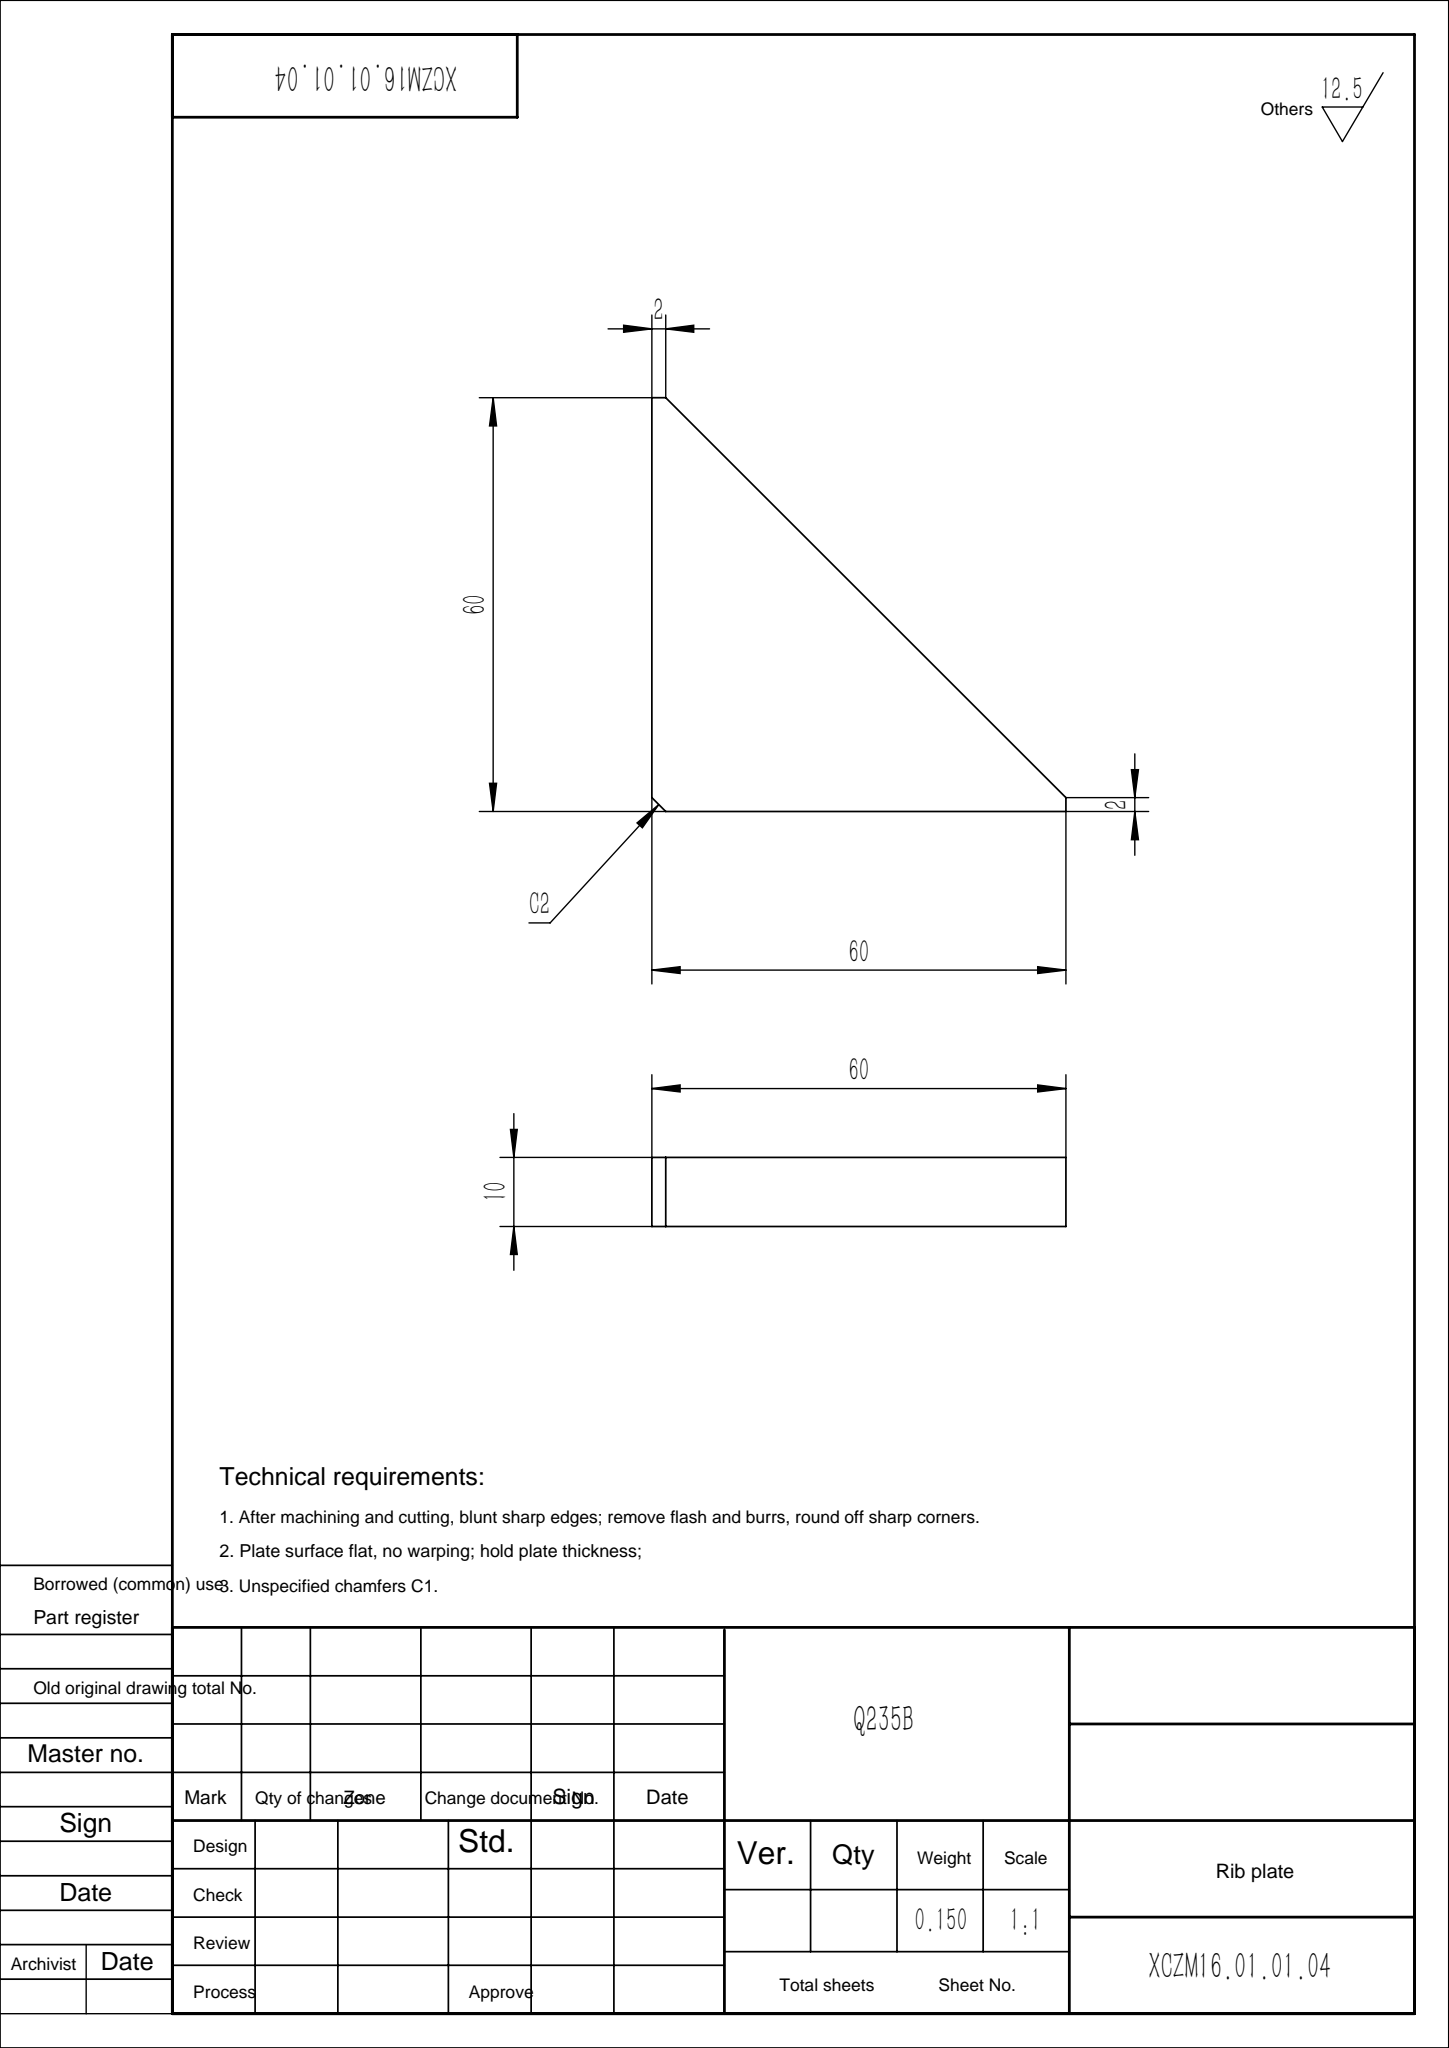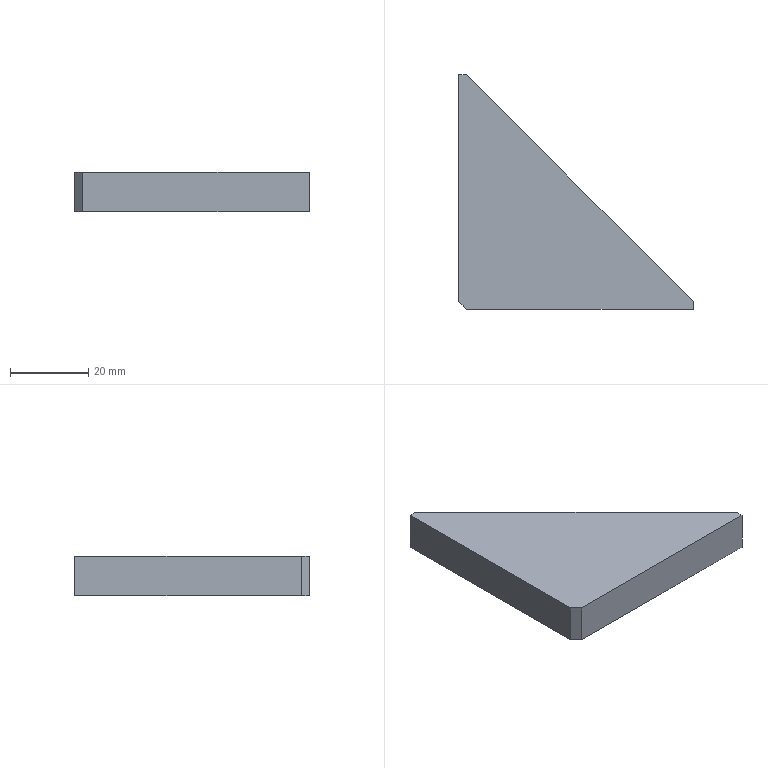Part | SolidWorks | features Chamfer 1, Extrusion 1 | 1 solid | 8 faces | box 60 x 60 x 10 mm | volume 19160 mm3 | plane 8
STEP:
#1=CARTESIAN_POINT('',(2.,60.,0.));
#2=VERTEX_POINT('',#1);
#3=CARTESIAN_POINT('',(0.,60.,0.));
#4=VERTEX_POINT('',#3);
#5=CARTESIAN_POINT('',(2.,60.,0.));
#6=DIRECTION('',(-1.,0.,0.));
#7=VECTOR('',#6,1000.);
#8=LINE('',#5,#7);
#9=EDGE_CURVE('',#2,#4,#8,.T.);
#10=ORIENTED_EDGE('',*,*,#9,.T.);
#11=CARTESIAN_POINT('',(0.,60.,10.));
#12=VERTEX_POINT('',#11);
#13=CARTESIAN_POINT('',(0.,60.,10.));
#14=DIRECTION('',(0.,0.,-1.));
#15=VECTOR('',#14,1000.);
#16=LINE('',#13,#15);
#17=EDGE_CURVE('',#12,#4,#16,.T.);
#18=ORIENTED_EDGE('',*,*,#17,.F.);
#19=CARTESIAN_POINT('',(2.,60.,10.));
#20=VERTEX_POINT('',#19);
#21=CARTESIAN_POINT('',(2.,60.,10.));
#22=DIRECTION('',(-1.,0.,0.));
#23=VECTOR('',#22,1000.);
#24=LINE('',#21,#23);
#25=EDGE_CURVE('',#20,#12,#24,.T.);
#26=ORIENTED_EDGE('',*,*,#25,.F.);
#27=CARTESIAN_POINT('',(2.,60.,10.));
#28=DIRECTION('',(0.,0.,-1.));
#29=VECTOR('',#28,1000.);
#30=LINE('',#27,#29);
#31=EDGE_CURVE('',#20,#2,#30,.T.);
#32=ORIENTED_EDGE('',*,*,#31,.T.);
#33=EDGE_LOOP('',(#10,#18,#26,#32));
#34=FACE_OUTER_BOUND('',#33,.T.);
#35=CARTESIAN_POINT('',(2.,60.,10.));
#36=DIRECTION('',(0.,-1.,0.));
#37=DIRECTION('',(0.,0.,-1.));
#38=AXIS2_PLACEMENT_3D('',#35,#36,#37);
#39=PLANE('',#38);
#40=ADVANCED_FACE('',(#34),#39,.F.);
#41=CARTESIAN_POINT('',(0.,2.,0.));
#42=VERTEX_POINT('',#41);
#43=CARTESIAN_POINT('',(0.,60.,0.));
#44=DIRECTION('',(0.,-1.,0.));
#45=VECTOR('',#44,1000.);
#46=LINE('',#43,#45);
#47=EDGE_CURVE('',#4,#42,#46,.T.);
#48=ORIENTED_EDGE('',*,*,#47,.T.);
#49=CARTESIAN_POINT('',(0.,2.,10.));
#50=VERTEX_POINT('',#49);
#51=CARTESIAN_POINT('',(0.,2.,10.));
#52=DIRECTION('',(0.,0.,1.));
#53=VECTOR('',#52,1000.);
#54=LINE('',#51,#53);
#55=EDGE_CURVE('',#42,#50,#54,.T.);
#56=ORIENTED_EDGE('',*,*,#55,.T.);
#57=CARTESIAN_POINT('',(0.,60.,10.));
#58=DIRECTION('',(0.,-1.,0.));
#59=VECTOR('',#58,1000.);
#60=LINE('',#57,#59);
#61=EDGE_CURVE('',#12,#50,#60,.T.);
#62=ORIENTED_EDGE('',*,*,#61,.F.);
#63=ORIENTED_EDGE('',*,*,#17,.T.);
#64=EDGE_LOOP('',(#48,#56,#62,#63));
#65=FACE_OUTER_BOUND('',#64,.T.);
#66=CARTESIAN_POINT('',(0.,60.,10.));
#67=DIRECTION('',(1.,0.,0.));
#68=DIRECTION('',(0.,1.,0.));
#69=AXIS2_PLACEMENT_3D('',#66,#67,#68);
#70=PLANE('',#69);
#71=ADVANCED_FACE('',(#65),#70,.F.);
#72=CARTESIAN_POINT('',(2.,0.,10.));
#73=VERTEX_POINT('',#72);
#74=CARTESIAN_POINT('',(60.,0.,10.));
#75=VERTEX_POINT('',#74);
#76=CARTESIAN_POINT('',(0.,0.,10.));
#77=DIRECTION('',(1.,0.,0.));
#78=VECTOR('',#77,1000.);
#79=LINE('',#76,#78);
#80=EDGE_CURVE('',#73,#75,#79,.T.);
#81=ORIENTED_EDGE('',*,*,#80,.F.);
#82=CARTESIAN_POINT('',(2.,0.,0.));
#83=VERTEX_POINT('',#82);
#84=CARTESIAN_POINT('',(2.,0.,10.));
#85=DIRECTION('',(0.,0.,-1.));
#86=VECTOR('',#85,1000.);
#87=LINE('',#84,#86);
#88=EDGE_CURVE('',#73,#83,#87,.T.);
#89=ORIENTED_EDGE('',*,*,#88,.T.);
#90=CARTESIAN_POINT('',(60.,0.,0.));
#91=VERTEX_POINT('',#90);
#92=CARTESIAN_POINT('',(0.,0.,0.));
#93=DIRECTION('',(1.,0.,0.));
#94=VECTOR('',#93,1000.);
#95=LINE('',#92,#94);
#96=EDGE_CURVE('',#83,#91,#95,.T.);
#97=ORIENTED_EDGE('',*,*,#96,.T.);
#98=CARTESIAN_POINT('',(60.,0.,10.));
#99=DIRECTION('',(0.,0.,-1.));
#100=VECTOR('',#99,1000.);
#101=LINE('',#98,#100);
#102=EDGE_CURVE('',#75,#91,#101,.T.);
#103=ORIENTED_EDGE('',*,*,#102,.F.);
#104=EDGE_LOOP('',(#81,#89,#97,#103));
#105=FACE_OUTER_BOUND('',#104,.T.);
#106=CARTESIAN_POINT('',(0.,0.,10.));
#107=DIRECTION('',(0.,1.,0.));
#108=DIRECTION('',(0.,0.,1.));
#109=AXIS2_PLACEMENT_3D('',#106,#107,#108);
#110=PLANE('',#109);
#111=ADVANCED_FACE('',(#105),#110,.F.);
#112=CARTESIAN_POINT('',(60.,2.,0.));
#113=VERTEX_POINT('',#112);
#114=CARTESIAN_POINT('',(60.,0.,0.));
#115=DIRECTION('',(0.,1.,0.));
#116=VECTOR('',#115,1000.);
#117=LINE('',#114,#116);
#118=EDGE_CURVE('',#91,#113,#117,.T.);
#119=ORIENTED_EDGE('',*,*,#118,.T.);
#120=CARTESIAN_POINT('',(60.,2.,10.));
#121=VERTEX_POINT('',#120);
#122=CARTESIAN_POINT('',(60.,2.,10.));
#123=DIRECTION('',(0.,0.,-1.));
#124=VECTOR('',#123,1000.);
#125=LINE('',#122,#124);
#126=EDGE_CURVE('',#121,#113,#125,.T.);
#127=ORIENTED_EDGE('',*,*,#126,.F.);
#128=CARTESIAN_POINT('',(60.,0.,10.));
#129=DIRECTION('',(0.,1.,0.));
#130=VECTOR('',#129,1000.);
#131=LINE('',#128,#130);
#132=EDGE_CURVE('',#75,#121,#131,.T.);
#133=ORIENTED_EDGE('',*,*,#132,.F.);
#134=ORIENTED_EDGE('',*,*,#102,.T.);
#135=EDGE_LOOP('',(#119,#127,#133,#134));
#136=FACE_OUTER_BOUND('',#135,.T.);
#137=CARTESIAN_POINT('',(60.,0.,10.));
#138=DIRECTION('',(-1.,0.,0.));
#139=DIRECTION('',(0.,0.,1.));
#140=AXIS2_PLACEMENT_3D('',#137,#138,#139);
#141=PLANE('',#140);
#142=ADVANCED_FACE('',(#136),#141,.F.);
#143=CARTESIAN_POINT('',(60.,2.,0.));
#144=DIRECTION('',(-0.7071,0.7071,0.));
#145=VECTOR('',#144,1000.);
#146=LINE('',#143,#145);
#147=EDGE_CURVE('',#113,#2,#146,.T.);
#148=ORIENTED_EDGE('',*,*,#147,.T.);
#149=ORIENTED_EDGE('',*,*,#31,.F.);
#150=CARTESIAN_POINT('',(60.,2.,10.));
#151=DIRECTION('',(-0.7071,0.7071,0.));
#152=VECTOR('',#151,1000.);
#153=LINE('',#150,#152);
#154=EDGE_CURVE('',#121,#20,#153,.T.);
#155=ORIENTED_EDGE('',*,*,#154,.F.);
#156=ORIENTED_EDGE('',*,*,#126,.T.);
#157=EDGE_LOOP('',(#148,#149,#155,#156));
#158=FACE_OUTER_BOUND('',#157,.T.);
#159=CARTESIAN_POINT('',(60.,2.,10.));
#160=DIRECTION('',(-0.7071,-0.7071,0.));
#161=DIRECTION('',(0.7071,-0.7071,0.));
#162=AXIS2_PLACEMENT_3D('',#159,#160,#161);
#163=PLANE('',#162);
#164=ADVANCED_FACE('',(#158),#163,.F.);
#165=ORIENTED_EDGE('',*,*,#61,.T.);
#166=CARTESIAN_POINT('',(1.,1.,10.));
#167=DIRECTION('',(0.7071,-0.7071,0.));
#168=VECTOR('',#167,1000.);
#169=LINE('',#166,#168);
#170=EDGE_CURVE('',#50,#73,#169,.T.);
#171=ORIENTED_EDGE('',*,*,#170,.T.);
#172=ORIENTED_EDGE('',*,*,#80,.T.);
#173=ORIENTED_EDGE('',*,*,#132,.T.);
#174=ORIENTED_EDGE('',*,*,#154,.T.);
#175=ORIENTED_EDGE('',*,*,#25,.T.);
#176=EDGE_LOOP('',(#165,#171,#172,#173,#174,#175));
#177=FACE_OUTER_BOUND('',#176,.T.);
#178=CARTESIAN_POINT('',(0.,0.,10.));
#179=DIRECTION('',(0.,0.,1.));
#180=DIRECTION('',(1.,0.,0.));
#181=AXIS2_PLACEMENT_3D('',#178,#179,#180);
#182=PLANE('',#181);
#183=ADVANCED_FACE('',(#177),#182,.T.);
#184=ORIENTED_EDGE('',*,*,#96,.F.);
#185=CARTESIAN_POINT('',(2.,0.,0.));
#186=DIRECTION('',(-0.7071,0.7071,0.));
#187=VECTOR('',#186,1000.);
#188=LINE('',#185,#187);
#189=EDGE_CURVE('',#83,#42,#188,.T.);
#190=ORIENTED_EDGE('',*,*,#189,.T.);
#191=ORIENTED_EDGE('',*,*,#47,.F.);
#192=ORIENTED_EDGE('',*,*,#9,.F.);
#193=ORIENTED_EDGE('',*,*,#147,.F.);
#194=ORIENTED_EDGE('',*,*,#118,.F.);
#195=EDGE_LOOP('',(#184,#190,#191,#192,#193,#194));
#196=FACE_OUTER_BOUND('',#195,.T.);
#197=CARTESIAN_POINT('',(0.,0.,0.));
#198=DIRECTION('',(0.,0.,1.));
#199=DIRECTION('',(1.,0.,0.));
#200=AXIS2_PLACEMENT_3D('',#197,#198,#199);
#201=PLANE('',#200);
#202=ADVANCED_FACE('',(#196),#201,.F.);
#203=ORIENTED_EDGE('',*,*,#170,.F.);
#204=ORIENTED_EDGE('',*,*,#55,.F.);
#205=ORIENTED_EDGE('',*,*,#189,.F.);
#206=ORIENTED_EDGE('',*,*,#88,.F.);
#207=EDGE_LOOP('',(#203,#204,#205,#206));
#208=FACE_OUTER_BOUND('',#207,.T.);
#209=CARTESIAN_POINT('',(2.,0.,10.));
#210=DIRECTION('',(0.7071,0.7071,0.));
#211=DIRECTION('',(0.,0.,-1.));
#212=AXIS2_PLACEMENT_3D('',#209,#210,#211);
#213=PLANE('',#212);
#214=ADVANCED_FACE('',(#208),#213,.F.);
#215=CLOSED_SHELL('',(#40,#71,#111,#142,#164,#183,#202,#214));
#216=MANIFOLD_SOLID_BREP('',#215);
#217=CARTESIAN_POINT('',(0.,0.,0.));
#218=DIRECTION('',(0.,0.,1.));
#219=DIRECTION('',(1.,0.,0.));
#220=AXIS2_PLACEMENT_3D('',#217,#218,#219);
#221=(LENGTH_UNIT()NAMED_UNIT(*)SI_UNIT(.MILLI.,.METRE.));
#222=UNCERTAINTY_MEASURE_WITH_UNIT(LENGTH_MEASURE(0.00001),#221,'','');
#223=(NAMED_UNIT(*)PLANE_ANGLE_UNIT()SI_UNIT($,.RADIAN.));
#224=(NAMED_UNIT(*)SI_UNIT($,.STERADIAN.)SOLID_ANGLE_UNIT());
#225=(GEOMETRIC_REPRESENTATION_CONTEXT(3)GLOBAL_UNCERTAINTY_ASSIGNED_CONTEXT((#222))GLOBAL_UNIT_ASSIGNED_CONTEXT((#221,#223,#224))REPRESENTATION_CONTEXT('',''));
#226=ADVANCED_BREP_SHAPE_REPRESENTATION('',(#216,#220),#225);